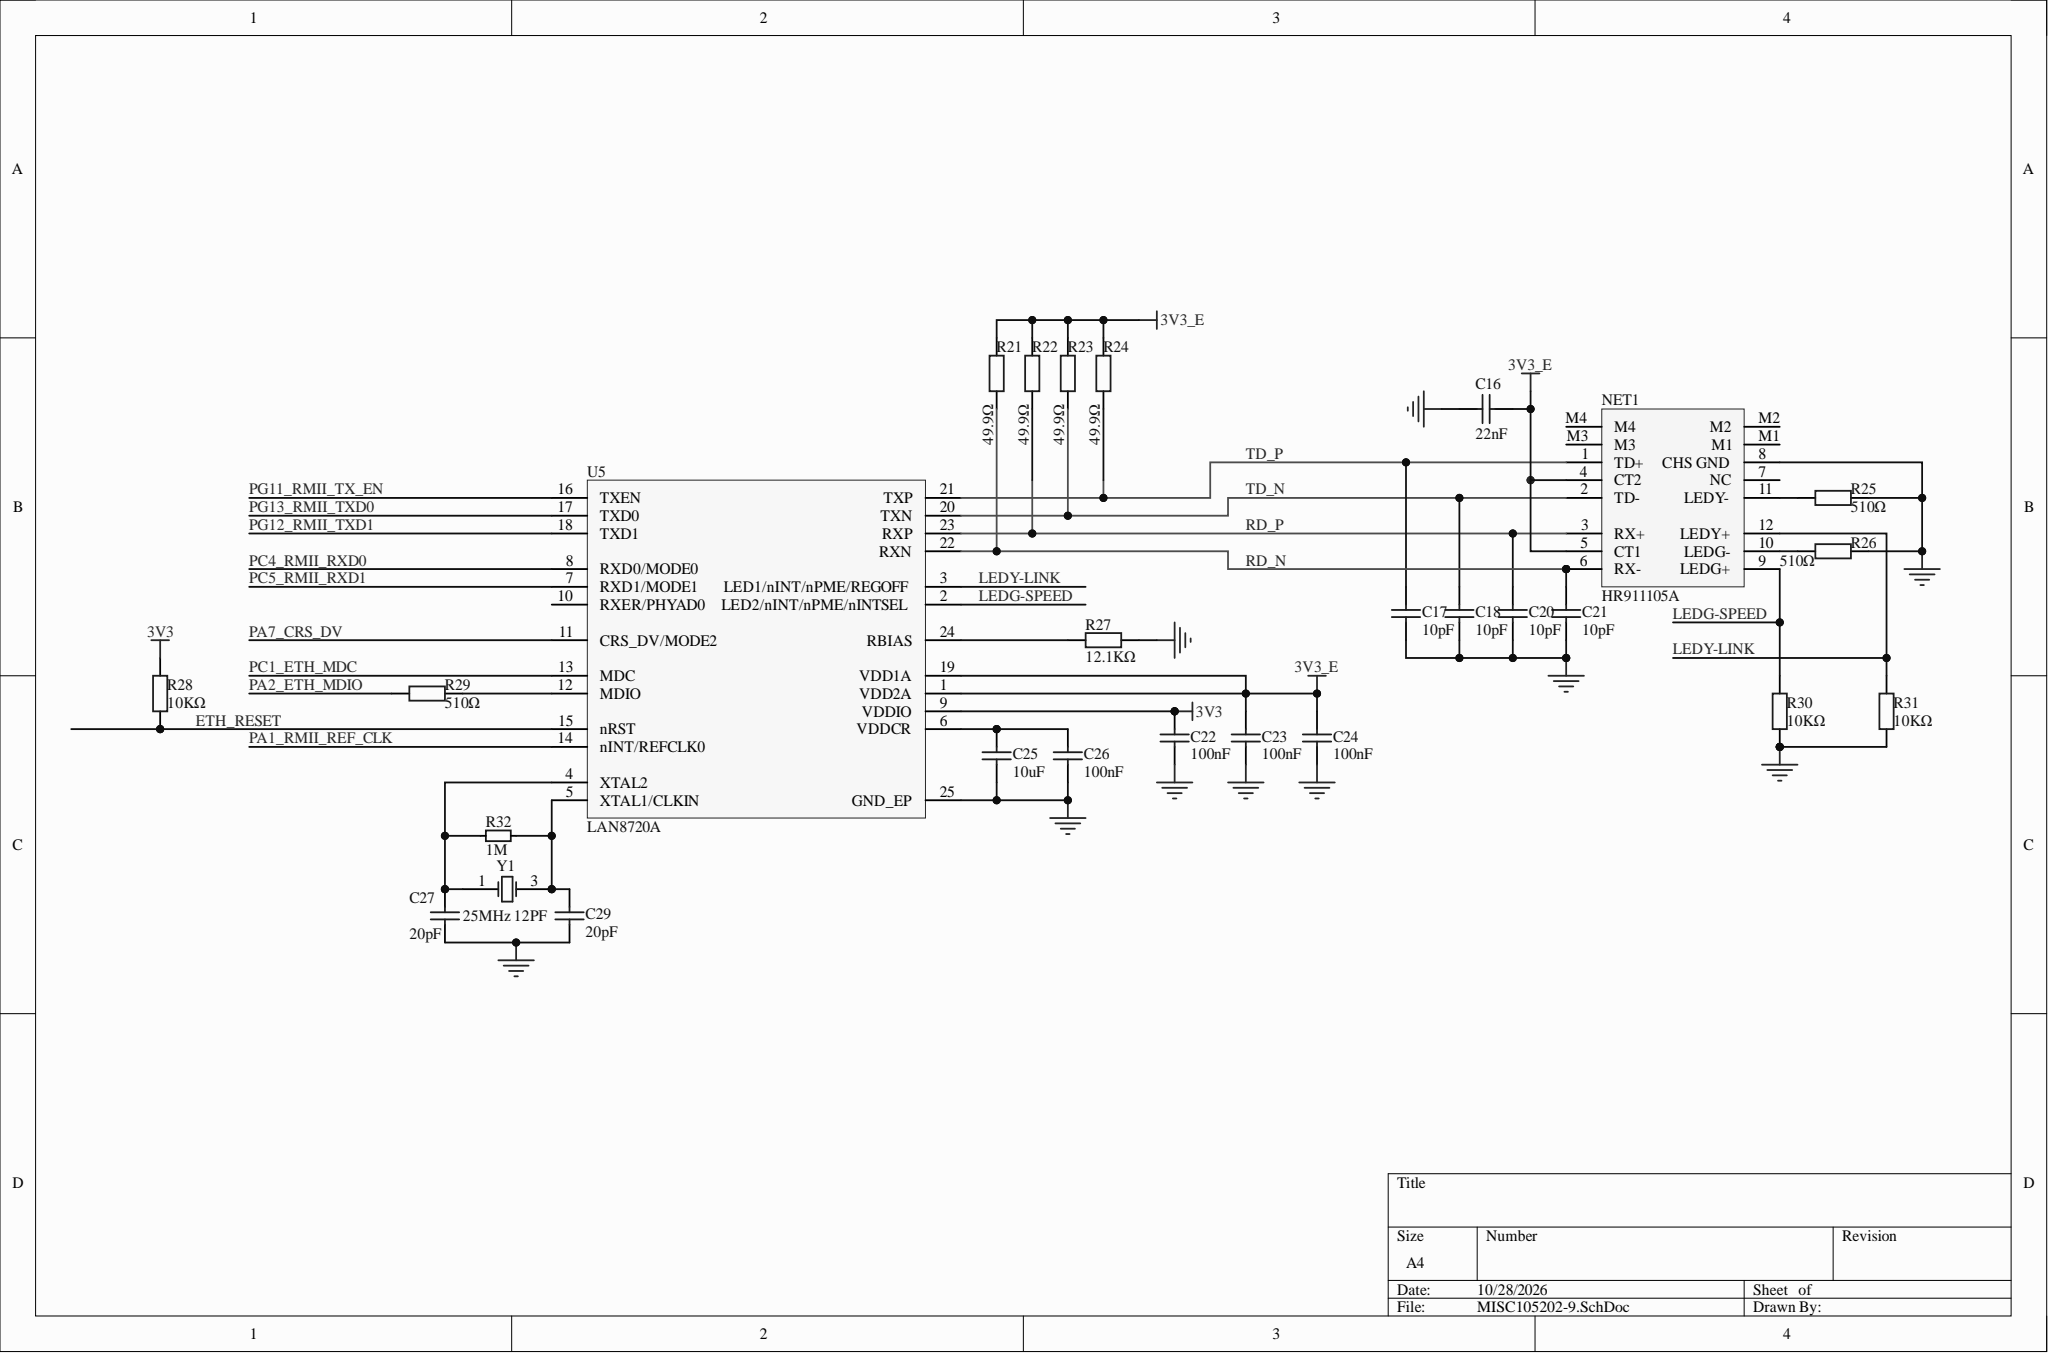Circuit board | Altium Designer | 181 parts | 141 nets | one sheet of the schematic
Parts on this sheet (reference | value | footprint):
C16 | 22nF | 0603_C
C17 | 10pF | 0603_C
C18 | 10pF | 0603_C
C20 | 10pF | 0603_C
C21 | 10pF | 0603_C
C22 | 100nF | 0603_C
C23 | 100nF | 0603_C
C24 | 100nF | 0603_C
C25 | 10uF | 0603_C
C26 | 100nF | 0603_C
C27 | 20pF | 0402_C
C29 | 20pF | 0402_C
NET1 | HR911105A | RJ45
R21 | 49.9Ω | 0603_R
R22 | 49.9Ω | 0603_R
R23 | 49.9Ω | 0603_R
R24 | 49.9Ω | 0603_R
R25 | 510Ω | 0603_R
R26 | 510Ω | 0603_R
R27 | 12.1KΩ | 0603_R
R28 | 10KΩ | 0603_R
R29 | 510Ω | 0603_R
R30 | 10KΩ | 0603_R
R31 | 10KΩ | 0603_R
R32 | 1M | 0402_R
U5 | LAN8720A | QFN-24_4X4x05P
Nets of these parts (net: part-pin ...):
TD_P: C17-1 NET1-1 R24-1 U5-21
TD_N: C18-1 NET1-2 R23-1 U5-20
RD_P: C20-1 NET1-3 R22-1 U5-23
RD_N: C21-1 NET1-6 R21-1 U5-22
PG13_RMII_TXD0: U5-17
PG12_RMII_TXD1: U5-18
PG11_RMII_TX_EN: U5-16
PC5_RMII_RXD1: U5-7
PC4_RMII_RXD0: U5-8
PC1_ETH_MDC: U5-13
PA7_CRS_DV: U5-11
PA2_ETH_MDIO: R29-1
PA1_RMII_REF_CLK: U5-14
NetR29_2: R29-2 U5-12
NetR27_1: R27-1 U5-24
NetNET1_11: NET1-11 R25-1
NetNET1_10: NET1-10 R26-1
NetC29_1: C29-1 R32-1 U5-5
NetC27_1: C27-1 R32-2 U5-4
NetC25_2: C25-2 C26-2 U5-6
LEDY-LINK: NET1-12 R31-2 U5-3
LEDG-SPEED: NET1-9 R30-1 U5-2
GND: C16-2 C17-2 C18-2 C20-2 C21-2 C22-1 C23-1 C24-1 C25-1 C26-1 C27-2 C29-2 NET1-8 R25-2 R26-2 R27-2 R30-2 R31-1 U5-25
ETH_RESET: R28-2 U5-15
3V3_E: C16-1 C23-2 C24-2 NET1-4 NET1-5 R21-2 R22-2 R23-2 R24-2 U5-1 U5-19
3V3: C22-2 R28-1 U5-9